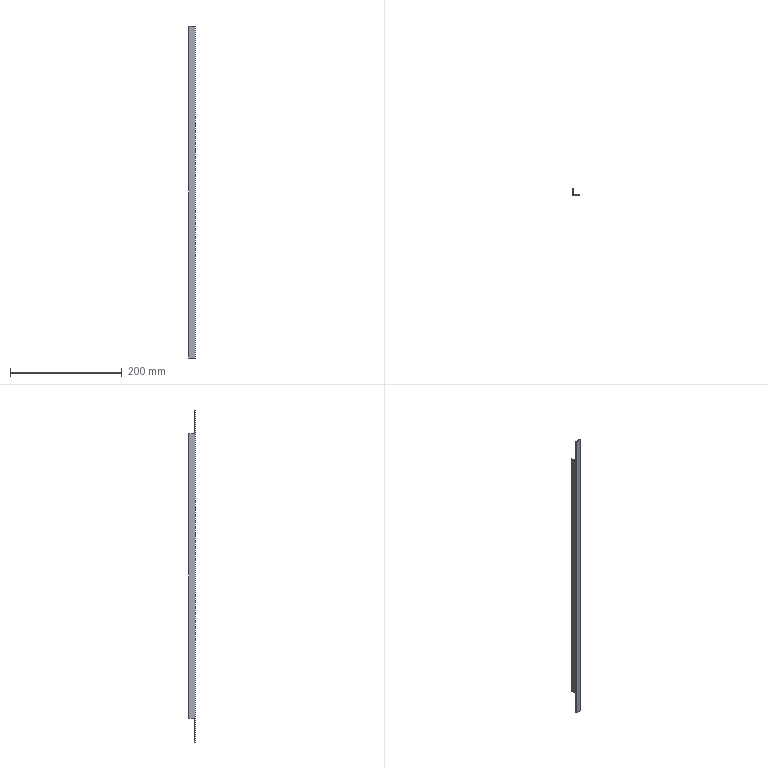Part | SolidWorks | features BaseBody 1 | 1 solid | 20 faces | box 12 x 12 x 594.4 mm | volume 15126 mm3 | plane 14 | cylinder 6 | commonest cylinder face diameters 0.6 x4 1 x2
STEP:
#1=CARTESIAN_POINT('',(1.2,1.7,297.2));
#2=VERTEX_POINT('',#1);
#3=CARTESIAN_POINT('',(1.7,1.2,297.2));
#4=VERTEX_POINT('',#3);
#5=CARTESIAN_POINT('',(1.7,1.7,297.2));
#6=DIRECTION('',(0.,0.,1.));
#7=DIRECTION('',(-1.,0.,0.));
#8=AXIS2_PLACEMENT_3D('',#5,#6,#7);
#9=CIRCLE('',#8,0.5);
#10=EDGE_CURVE('',#2,#4,#9,.T.);
#11=ORIENTED_EDGE('',*,*,#10,.T.);
#12=CARTESIAN_POINT('',(1.7,1.2,-297.2));
#13=VERTEX_POINT('',#12);
#14=CARTESIAN_POINT('',(1.7,1.2,0.));
#15=DIRECTION('',(0.,0.,-1.));
#16=VECTOR('',#15,1000.);
#17=LINE('',#14,#16);
#18=EDGE_CURVE('',#4,#13,#17,.T.);
#19=ORIENTED_EDGE('',*,*,#18,.T.);
#20=CARTESIAN_POINT('',(1.2,1.7,-297.2));
#21=VERTEX_POINT('',#20);
#22=CARTESIAN_POINT('',(1.7,1.7,-297.2));
#23=DIRECTION('',(0.,0.,1.));
#24=DIRECTION('',(-1.,0.,0.));
#25=AXIS2_PLACEMENT_3D('',#22,#23,#24);
#26=CIRCLE('',#25,0.5);
#27=EDGE_CURVE('',#21,#13,#26,.T.);
#28=ORIENTED_EDGE('',*,*,#27,.F.);
#29=CARTESIAN_POINT('',(1.2,1.7,-255.));
#30=VERTEX_POINT('',#29);
#31=CARTESIAN_POINT('',(1.2,1.7,0.));
#32=DIRECTION('',(0.,0.,1.));
#33=VECTOR('',#32,1000.);
#34=LINE('',#31,#33);
#35=EDGE_CURVE('',#21,#30,#34,.T.);
#36=ORIENTED_EDGE('',*,*,#35,.T.);
#37=CARTESIAN_POINT('',(1.2,1.7,255.));
#38=VERTEX_POINT('',#37);
#39=CARTESIAN_POINT('',(1.2,1.7,0.));
#40=DIRECTION('',(0.,0.,1.));
#41=VECTOR('',#40,1000.);
#42=LINE('',#39,#41);
#43=EDGE_CURVE('',#30,#38,#42,.T.);
#44=ORIENTED_EDGE('',*,*,#43,.T.);
#45=CARTESIAN_POINT('',(1.2,1.7,0.));
#46=DIRECTION('',(0.,0.,1.));
#47=VECTOR('',#46,1000.);
#48=LINE('',#45,#47);
#49=EDGE_CURVE('',#38,#2,#48,.T.);
#50=ORIENTED_EDGE('',*,*,#49,.T.);
#51=EDGE_LOOP('',(#11,#19,#28,#36,#44,#50));
#52=FACE_OUTER_BOUND('',#51,.T.);
#53=CARTESIAN_POINT('',(1.7,1.7,297.2));
#54=DIRECTION('',(0.,0.,-1.));
#55=DIRECTION('',(-1.,0.,0.));
#56=AXIS2_PLACEMENT_3D('',#53,#54,#55);
#57=CYLINDRICAL_SURFACE('',#56,0.5);
#58=ADVANCED_FACE('',(#52),#57,.F.);
#59=ORIENTED_EDGE('',*,*,#18,.F.);
#60=CARTESIAN_POINT('',(11.7,1.2,297.2));
#61=VERTEX_POINT('',#60);
#62=CARTESIAN_POINT('',(6.7,1.2,297.2));
#63=DIRECTION('',(-1.,0.,0.));
#64=VECTOR('',#63,1000.);
#65=LINE('',#62,#64);
#66=EDGE_CURVE('',#61,#4,#65,.T.);
#67=ORIENTED_EDGE('',*,*,#66,.F.);
#68=CARTESIAN_POINT('',(11.7,1.2,-297.2));
#69=VERTEX_POINT('',#68);
#70=CARTESIAN_POINT('',(11.7,1.2,0.));
#71=DIRECTION('',(0.,0.,1.));
#72=VECTOR('',#71,1000.);
#73=LINE('',#70,#72);
#74=EDGE_CURVE('',#69,#61,#73,.T.);
#75=ORIENTED_EDGE('',*,*,#74,.F.);
#76=CARTESIAN_POINT('',(6.7,1.2,-297.2));
#77=DIRECTION('',(1.,0.,0.));
#78=VECTOR('',#77,1000.);
#79=LINE('',#76,#78);
#80=EDGE_CURVE('',#13,#69,#79,.T.);
#81=ORIENTED_EDGE('',*,*,#80,.F.);
#82=EDGE_LOOP('',(#59,#67,#75,#81));
#83=FACE_OUTER_BOUND('',#82,.T.);
#84=CARTESIAN_POINT('',(1.7,1.2,-297.2));
#85=DIRECTION('',(0.,-1.,0.));
#86=DIRECTION('',(1.,0.,0.));
#87=AXIS2_PLACEMENT_3D('',#84,#85,#86);
#88=PLANE('',#87);
#89=ADVANCED_FACE('',(#83),#88,.F.);
#90=CARTESIAN_POINT('',(1.2,1.2,297.2));
#91=VERTEX_POINT('',#90);
#92=CARTESIAN_POINT('',(1.2,1.2,255.));
#93=VERTEX_POINT('',#92);
#94=CARTESIAN_POINT('',(1.2,1.2,276.1));
#95=DIRECTION('',(0.,0.,-1.));
#96=VECTOR('',#95,1000.);
#97=LINE('',#94,#96);
#98=EDGE_CURVE('',#91,#93,#97,.T.);
#99=ORIENTED_EDGE('',*,*,#98,.F.);
#100=CARTESIAN_POINT('',(1.2,1.45,297.2));
#101=DIRECTION('',(0.,-1.,0.));
#102=VECTOR('',#101,1000.);
#103=LINE('',#100,#102);
#104=EDGE_CURVE('',#2,#91,#103,.T.);
#105=ORIENTED_EDGE('',*,*,#104,.F.);
#106=ORIENTED_EDGE('',*,*,#49,.F.);
#107=CARTESIAN_POINT('',(1.2,6.6,255.));
#108=DIRECTION('',(0.,-1.,0.));
#109=VECTOR('',#108,1000.);
#110=LINE('',#107,#109);
#111=EDGE_CURVE('',#38,#93,#110,.T.);
#112=ORIENTED_EDGE('',*,*,#111,.T.);
#113=EDGE_LOOP('',(#99,#105,#106,#112));
#114=FACE_OUTER_BOUND('',#113,.T.);
#115=CARTESIAN_POINT('',(1.2,1.2,255.));
#116=DIRECTION('',(1.,0.,0.));
#117=DIRECTION('',(0.,1.,0.));
#118=AXIS2_PLACEMENT_3D('',#115,#116,#117);
#119=PLANE('',#118);
#120=ADVANCED_FACE('',(#114),#119,.F.);
#121=CARTESIAN_POINT('',(1.2,11.7,-255.));
#122=VERTEX_POINT('',#121);
#123=CARTESIAN_POINT('',(1.2,6.7,-255.));
#124=DIRECTION('',(0.,-1.,0.));
#125=VECTOR('',#124,1000.);
#126=LINE('',#123,#125);
#127=EDGE_CURVE('',#122,#30,#126,.T.);
#128=ORIENTED_EDGE('',*,*,#127,.F.);
#129=CARTESIAN_POINT('',(1.2,11.7,255.));
#130=VERTEX_POINT('',#129);
#131=CARTESIAN_POINT('',(1.2,11.7,0.));
#132=DIRECTION('',(0.,0.,-1.));
#133=VECTOR('',#132,1000.);
#134=LINE('',#131,#133);
#135=EDGE_CURVE('',#130,#122,#134,.T.);
#136=ORIENTED_EDGE('',*,*,#135,.F.);
#137=CARTESIAN_POINT('',(1.2,6.7,255.));
#138=DIRECTION('',(0.,1.,0.));
#139=VECTOR('',#138,1000.);
#140=LINE('',#137,#139);
#141=EDGE_CURVE('',#38,#130,#140,.T.);
#142=ORIENTED_EDGE('',*,*,#141,.F.);
#143=ORIENTED_EDGE('',*,*,#43,.F.);
#144=EDGE_LOOP('',(#128,#136,#142,#143));
#145=FACE_OUTER_BOUND('',#144,.T.);
#146=CARTESIAN_POINT('',(1.2,11.7,-255.));
#147=DIRECTION('',(-1.,0.,0.));
#148=DIRECTION('',(0.,-1.,0.));
#149=AXIS2_PLACEMENT_3D('',#146,#147,#148);
#150=PLANE('',#149);
#151=ADVANCED_FACE('',(#145),#150,.F.);
#152=CARTESIAN_POINT('',(1.2,1.2,-255.));
#153=VERTEX_POINT('',#152);
#154=CARTESIAN_POINT('',(1.2,1.2,-297.2));
#155=VERTEX_POINT('',#154);
#156=CARTESIAN_POINT('',(1.2,1.2,-276.1));
#157=DIRECTION('',(0.,0.,-1.));
#158=VECTOR('',#157,1000.);
#159=LINE('',#156,#158);
#160=EDGE_CURVE('',#153,#155,#159,.T.);
#161=ORIENTED_EDGE('',*,*,#160,.F.);
#162=CARTESIAN_POINT('',(1.2,1.45,-255.));
#163=DIRECTION('',(0.,-1.,0.));
#164=VECTOR('',#163,1000.);
#165=LINE('',#162,#164);
#166=EDGE_CURVE('',#30,#153,#165,.T.);
#167=ORIENTED_EDGE('',*,*,#166,.F.);
#168=ORIENTED_EDGE('',*,*,#35,.F.);
#169=CARTESIAN_POINT('',(1.2,1.45,-297.2));
#170=DIRECTION('',(0.,1.,0.));
#171=VECTOR('',#170,1000.);
#172=LINE('',#169,#171);
#173=EDGE_CURVE('',#155,#21,#172,.T.);
#174=ORIENTED_EDGE('',*,*,#173,.F.);
#175=EDGE_LOOP('',(#161,#167,#168,#174));
#176=FACE_OUTER_BOUND('',#175,.T.);
#177=CARTESIAN_POINT('',(1.2,1.2,-297.2));
#178=DIRECTION('',(1.,0.,0.));
#179=DIRECTION('',(0.,1.,0.));
#180=AXIS2_PLACEMENT_3D('',#177,#178,#179);
#181=PLANE('',#180);
#182=ADVANCED_FACE('',(#176),#181,.F.);
#183=CARTESIAN_POINT('',(0.5,0.,-297.2));
#184=VERTEX_POINT('',#183);
#185=CARTESIAN_POINT('',(0.,0.5,-297.2));
#186=VERTEX_POINT('',#185);
#187=CARTESIAN_POINT('',(0.5,0.5,-297.2));
#188=DIRECTION('',(0.,0.,-1.));
#189=DIRECTION('',(-1.,0.,0.));
#190=AXIS2_PLACEMENT_3D('',#187,#188,#189);
#191=CIRCLE('',#190,0.5);
#192=EDGE_CURVE('',#184,#186,#191,.T.);
#193=ORIENTED_EDGE('',*,*,#192,.T.);
#194=CARTESIAN_POINT('',(0.,1.2,-297.2));
#195=VERTEX_POINT('',#194);
#196=CARTESIAN_POINT('',(0.,6.1,-297.2));
#197=DIRECTION('',(0.,1.,0.));
#198=VECTOR('',#197,1000.);
#199=LINE('',#196,#198);
#200=EDGE_CURVE('',#186,#195,#199,.T.);
#201=ORIENTED_EDGE('',*,*,#200,.T.);
#202=CARTESIAN_POINT('',(6.,1.2,-297.2));
#203=DIRECTION('',(1.,0.,0.));
#204=VECTOR('',#203,1000.);
#205=LINE('',#202,#204);
#206=EDGE_CURVE('',#195,#155,#205,.T.);
#207=ORIENTED_EDGE('',*,*,#206,.T.);
#208=ORIENTED_EDGE('',*,*,#173,.T.);
#209=ORIENTED_EDGE('',*,*,#27,.T.);
#210=ORIENTED_EDGE('',*,*,#80,.T.);
#211=CARTESIAN_POINT('',(12.,0.9,-297.2));
#212=VERTEX_POINT('',#211);
#213=CARTESIAN_POINT('',(11.7,0.9,-297.2));
#214=DIRECTION('',(0.,0.,-1.));
#215=DIRECTION('',(-1.,0.,0.));
#216=AXIS2_PLACEMENT_3D('',#213,#214,#215);
#217=CIRCLE('',#216,0.3);
#218=EDGE_CURVE('',#69,#212,#217,.T.);
#219=ORIENTED_EDGE('',*,*,#218,.T.);
#220=CARTESIAN_POINT('',(12.,0.3,-297.2));
#221=VERTEX_POINT('',#220);
#222=CARTESIAN_POINT('',(12.,0.6,-297.2));
#223=DIRECTION('',(0.,-1.,0.));
#224=VECTOR('',#223,1000.);
#225=LINE('',#222,#224);
#226=EDGE_CURVE('',#212,#221,#225,.T.);
#227=ORIENTED_EDGE('',*,*,#226,.T.);
#228=CARTESIAN_POINT('',(11.7,0.,-297.2));
#229=VERTEX_POINT('',#228);
#230=CARTESIAN_POINT('',(11.7,0.3,-297.2));
#231=DIRECTION('',(0.,0.,-1.));
#232=DIRECTION('',(-1.,0.,0.));
#233=AXIS2_PLACEMENT_3D('',#230,#231,#232);
#234=CIRCLE('',#233,0.3);
#235=EDGE_CURVE('',#221,#229,#234,.T.);
#236=ORIENTED_EDGE('',*,*,#235,.T.);
#237=CARTESIAN_POINT('',(6.,0.,-297.2));
#238=DIRECTION('',(-1.,0.,0.));
#239=VECTOR('',#238,1000.);
#240=LINE('',#237,#239);
#241=EDGE_CURVE('',#229,#184,#240,.T.);
#242=ORIENTED_EDGE('',*,*,#241,.T.);
#243=EDGE_LOOP('',(#193,#201,#207,#208,#209,#210,#219,#227,#236,#242));
#244=FACE_OUTER_BOUND('',#243,.T.);
#245=CARTESIAN_POINT('',(12.,0.,-297.2));
#246=DIRECTION('',(0.,0.,-1.));
#247=DIRECTION('',(-1.,0.,0.));
#248=AXIS2_PLACEMENT_3D('',#245,#246,#247);
#249=PLANE('',#248);
#250=ADVANCED_FACE('',(#244),#249,.T.);
#251=CARTESIAN_POINT('',(0.,1.2,297.2));
#252=VERTEX_POINT('',#251);
#253=CARTESIAN_POINT('',(6.,1.2,297.2));
#254=DIRECTION('',(1.,0.,0.));
#255=VECTOR('',#254,1000.);
#256=LINE('',#253,#255);
#257=EDGE_CURVE('',#252,#91,#256,.T.);
#258=ORIENTED_EDGE('',*,*,#257,.F.);
#259=CARTESIAN_POINT('',(0.,0.5,297.2));
#260=VERTEX_POINT('',#259);
#261=CARTESIAN_POINT('',(0.,6.1,297.2));
#262=DIRECTION('',(0.,-1.,0.));
#263=VECTOR('',#262,1000.);
#264=LINE('',#261,#263);
#265=EDGE_CURVE('',#252,#260,#264,.T.);
#266=ORIENTED_EDGE('',*,*,#265,.T.);
#267=CARTESIAN_POINT('',(0.5,0.,297.2));
#268=VERTEX_POINT('',#267);
#269=CARTESIAN_POINT('',(0.5,0.5,297.2));
#270=DIRECTION('',(0.,0.,1.));
#271=DIRECTION('',(-1.,0.,0.));
#272=AXIS2_PLACEMENT_3D('',#269,#270,#271);
#273=CIRCLE('',#272,0.5);
#274=EDGE_CURVE('',#260,#268,#273,.T.);
#275=ORIENTED_EDGE('',*,*,#274,.T.);
#276=CARTESIAN_POINT('',(11.7,0.,297.2));
#277=VERTEX_POINT('',#276);
#278=CARTESIAN_POINT('',(6.,0.,297.2));
#279=DIRECTION('',(-1.,0.,0.));
#280=VECTOR('',#279,1000.);
#281=LINE('',#278,#280);
#282=EDGE_CURVE('',#277,#268,#281,.T.);
#283=ORIENTED_EDGE('',*,*,#282,.F.);
#284=CARTESIAN_POINT('',(12.,0.3,297.2));
#285=VERTEX_POINT('',#284);
#286=CARTESIAN_POINT('',(11.7,0.3,297.2));
#287=DIRECTION('',(0.,0.,1.));
#288=DIRECTION('',(-1.,0.,0.));
#289=AXIS2_PLACEMENT_3D('',#286,#287,#288);
#290=CIRCLE('',#289,0.3);
#291=EDGE_CURVE('',#277,#285,#290,.T.);
#292=ORIENTED_EDGE('',*,*,#291,.T.);
#293=CARTESIAN_POINT('',(12.,0.9,297.2));
#294=VERTEX_POINT('',#293);
#295=CARTESIAN_POINT('',(12.,0.6,297.2));
#296=DIRECTION('',(0.,1.,0.));
#297=VECTOR('',#296,1000.);
#298=LINE('',#295,#297);
#299=EDGE_CURVE('',#285,#294,#298,.T.);
#300=ORIENTED_EDGE('',*,*,#299,.T.);
#301=CARTESIAN_POINT('',(11.7,0.9,297.2));
#302=DIRECTION('',(0.,0.,-1.));
#303=DIRECTION('',(-1.,0.,0.));
#304=AXIS2_PLACEMENT_3D('',#301,#302,#303);
#305=CIRCLE('',#304,0.3);
#306=EDGE_CURVE('',#61,#294,#305,.T.);
#307=ORIENTED_EDGE('',*,*,#306,.F.);
#308=ORIENTED_EDGE('',*,*,#66,.T.);
#309=ORIENTED_EDGE('',*,*,#10,.F.);
#310=ORIENTED_EDGE('',*,*,#104,.T.);
#311=EDGE_LOOP('',(#258,#266,#275,#283,#292,#300,#307,#308,#309,#310));
#312=FACE_OUTER_BOUND('',#311,.T.);
#313=CARTESIAN_POINT('',(12.,0.,297.2));
#314=DIRECTION('',(0.,0.,-1.));
#315=DIRECTION('',(-1.,0.,0.));
#316=AXIS2_PLACEMENT_3D('',#313,#314,#315);
#317=PLANE('',#316);
#318=ADVANCED_FACE('',(#312),#317,.F.);
#319=ORIENTED_EDGE('',*,*,#74,.T.);
#320=ORIENTED_EDGE('',*,*,#306,.T.);
#321=CARTESIAN_POINT('',(12.,0.9,0.));
#322=DIRECTION('',(0.,0.,1.));
#323=VECTOR('',#322,1000.);
#324=LINE('',#321,#323);
#325=EDGE_CURVE('',#212,#294,#324,.T.);
#326=ORIENTED_EDGE('',*,*,#325,.F.);
#327=ORIENTED_EDGE('',*,*,#218,.F.);
#328=EDGE_LOOP('',(#319,#320,#326,#327));
#329=FACE_OUTER_BOUND('',#328,.T.);
#330=CARTESIAN_POINT('',(11.7,0.9,297.2));
#331=DIRECTION('',(0.,0.,-1.));
#332=DIRECTION('',(-1.,0.,0.));
#333=AXIS2_PLACEMENT_3D('',#330,#331,#332);
#334=CYLINDRICAL_SURFACE('',#333,0.3);
#335=ADVANCED_FACE('',(#329),#334,.T.);
#336=ORIENTED_EDGE('',*,*,#98,.T.);
#337=CARTESIAN_POINT('',(0.,1.2,255.));
#338=VERTEX_POINT('',#337);
#339=CARTESIAN_POINT('',(0.6,1.2,255.));
#340=DIRECTION('',(1.,0.,0.));
#341=VECTOR('',#340,1000.);
#342=LINE('',#339,#341);
#343=EDGE_CURVE('',#338,#93,#342,.T.);
#344=ORIENTED_EDGE('',*,*,#343,.F.);
#345=CARTESIAN_POINT('',(0.,1.2,276.1));
#346=DIRECTION('',(0.,0.,-1.));
#347=VECTOR('',#346,1000.);
#348=LINE('',#345,#347);
#349=EDGE_CURVE('',#252,#338,#348,.T.);
#350=ORIENTED_EDGE('',*,*,#349,.F.);
#351=ORIENTED_EDGE('',*,*,#257,.T.);
#352=EDGE_LOOP('',(#336,#344,#350,#351));
#353=FACE_OUTER_BOUND('',#352,.T.);
#354=CARTESIAN_POINT('',(0.,1.2,255.));
#355=DIRECTION('',(0.,-1.,0.));
#356=DIRECTION('',(1.,0.,0.));
#357=AXIS2_PLACEMENT_3D('',#354,#355,#356);
#358=PLANE('',#357);
#359=ADVANCED_FACE('',(#353),#358,.F.);
#360=ORIENTED_EDGE('',*,*,#166,.T.);
#361=CARTESIAN_POINT('',(0.,1.2,-255.));
#362=VERTEX_POINT('',#361);
#363=CARTESIAN_POINT('',(0.6,1.2,-255.));
#364=DIRECTION('',(1.,0.,0.));
#365=VECTOR('',#364,1000.);
#366=LINE('',#363,#365);
#367=EDGE_CURVE('',#362,#153,#366,.T.);
#368=ORIENTED_EDGE('',*,*,#367,.F.);
#369=CARTESIAN_POINT('',(0.,11.7,-255.));
#370=VERTEX_POINT('',#369);
#371=CARTESIAN_POINT('',(0.,6.6,-255.));
#372=DIRECTION('',(0.,-1.,0.));
#373=VECTOR('',#372,1000.);
#374=LINE('',#371,#373);
#375=EDGE_CURVE('',#370,#362,#374,.T.);
#376=ORIENTED_EDGE('',*,*,#375,.F.);
#377=CARTESIAN_POINT('',(0.3,12.,-255.));
#378=VERTEX_POINT('',#377);
#379=CARTESIAN_POINT('',(0.3,11.7,-255.));
#380=DIRECTION('',(0.,0.,-1.));
#381=DIRECTION('',(-1.,0.,0.));
#382=AXIS2_PLACEMENT_3D('',#379,#380,#381);
#383=CIRCLE('',#382,0.3);
#384=EDGE_CURVE('',#370,#378,#383,.T.);
#385=ORIENTED_EDGE('',*,*,#384,.T.);
#386=CARTESIAN_POINT('',(0.9,12.,-255.));
#387=VERTEX_POINT('',#386);
#388=CARTESIAN_POINT('',(0.6,12.,-255.));
#389=DIRECTION('',(1.,0.,0.));
#390=VECTOR('',#389,1000.);
#391=LINE('',#388,#390);
#392=EDGE_CURVE('',#378,#387,#391,.T.);
#393=ORIENTED_EDGE('',*,*,#392,.T.);
#394=CARTESIAN_POINT('',(0.9,11.7,-255.));
#395=DIRECTION('',(0.,0.,1.));
#396=DIRECTION('',(-1.,0.,0.));
#397=AXIS2_PLACEMENT_3D('',#394,#395,#396);
#398=CIRCLE('',#397,0.3);
#399=EDGE_CURVE('',#122,#387,#398,.T.);
#400=ORIENTED_EDGE('',*,*,#399,.F.);
#401=ORIENTED_EDGE('',*,*,#127,.T.);
#402=EDGE_LOOP('',(#360,#368,#376,#385,#393,#400,#401));
#403=FACE_OUTER_BOUND('',#402,.T.);
#404=CARTESIAN_POINT('',(0.,1.2,-255.));
#405=DIRECTION('',(0.,0.,1.));
#406=DIRECTION('',(1.,0.,0.));
#407=AXIS2_PLACEMENT_3D('',#404,#405,#406);
#408=PLANE('',#407);
#409=ADVANCED_FACE('',(#403),#408,.F.);
#410=ORIENTED_EDGE('',*,*,#399,.T.);
#411=CARTESIAN_POINT('',(0.9,12.,255.));
#412=VERTEX_POINT('',#411);
#413=CARTESIAN_POINT('',(0.9,12.,0.));
#414=DIRECTION('',(0.,0.,-1.));
#415=VECTOR('',#414,1000.);
#416=LINE('',#413,#415);
#417=EDGE_CURVE('',#412,#387,#416,.T.);
#418=ORIENTED_EDGE('',*,*,#417,.F.);
#419=CARTESIAN_POINT('',(0.9,11.7,255.));
#420=DIRECTION('',(0.,0.,1.));
#421=DIRECTION('',(-1.,0.,0.));
#422=AXIS2_PLACEMENT_3D('',#419,#420,#421);
#423=CIRCLE('',#422,0.3);
#424=EDGE_CURVE('',#130,#412,#423,.T.);
#425=ORIENTED_EDGE('',*,*,#424,.F.);
#426=ORIENTED_EDGE('',*,*,#135,.T.);
#427=EDGE_LOOP('',(#410,#418,#425,#426));
#428=FACE_OUTER_BOUND('',#427,.T.);
#429=CARTESIAN_POINT('',(0.9,11.7,255.));
#430=DIRECTION('',(0.,0.,-1.));
#431=DIRECTION('',(-1.,0.,0.));
#432=AXIS2_PLACEMENT_3D('',#429,#430,#431);
#433=CYLINDRICAL_SURFACE('',#432,0.3);
#434=ADVANCED_FACE('',(#428),#433,.T.);
#435=CARTESIAN_POINT('',(0.3,12.,255.));
#436=VERTEX_POINT('',#435);
#437=CARTESIAN_POINT('',(0.,11.7,255.));
#438=VERTEX_POINT('',#437);
#439=CARTESIAN_POINT('',(0.3,11.7,255.));
#440=DIRECTION('',(0.,0.,1.));
#441=DIRECTION('',(-1.,0.,0.));
#442=AXIS2_PLACEMENT_3D('',#439,#440,#441);
#443=CIRCLE('',#442,0.3);
#444=EDGE_CURVE('',#436,#438,#443,.T.);
#445=ORIENTED_EDGE('',*,*,#444,.T.);
#446=CARTESIAN_POINT('',(0.,6.6,255.));
#447=DIRECTION('',(0.,1.,0.));
#448=VECTOR('',#447,1000.);
#449=LINE('',#446,#448);
#450=EDGE_CURVE('',#338,#438,#449,.T.);
#451=ORIENTED_EDGE('',*,*,#450,.F.);
#452=ORIENTED_EDGE('',*,*,#343,.T.);
#453=ORIENTED_EDGE('',*,*,#111,.F.);
#454=ORIENTED_EDGE('',*,*,#141,.T.);
#455=ORIENTED_EDGE('',*,*,#424,.T.);
#456=CARTESIAN_POINT('',(0.6,12.,255.));
#457=DIRECTION('',(1.,0.,0.));
#458=VECTOR('',#457,1000.);
#459=LINE('',#456,#458);
#460=EDGE_CURVE('',#436,#412,#459,.T.);
#461=ORIENTED_EDGE('',*,*,#460,.F.);
#462=EDGE_LOOP('',(#445,#451,#452,#453,#454,#455,#461));
#463=FACE_OUTER_BOUND('',#462,.T.);
#464=CARTESIAN_POINT('',(1.2,1.2,255.));
#465=DIRECTION('',(0.,0.,-1.));
#466=DIRECTION('',(-1.,0.,0.));
#467=AXIS2_PLACEMENT_3D('',#464,#465,#466);
#468=PLANE('',#467);
#469=ADVANCED_FACE('',(#463),#468,.F.);
#470=ORIENTED_EDGE('',*,*,#160,.T.);
#471=ORIENTED_EDGE('',*,*,#206,.F.);
#472=CARTESIAN_POINT('',(0.,1.2,-276.1));
#473=DIRECTION('',(0.,0.,-1.));
#474=VECTOR('',#473,1000.);
#475=LINE('',#472,#474);
#476=EDGE_CURVE('',#362,#195,#475,.T.);
#477=ORIENTED_EDGE('',*,*,#476,.F.);
#478=ORIENTED_EDGE('',*,*,#367,.T.);
#479=EDGE_LOOP('',(#470,#471,#477,#478));
#480=FACE_OUTER_BOUND('',#479,.T.);
#481=CARTESIAN_POINT('',(0.,1.2,-297.2));
#482=DIRECTION('',(0.,-1.,0.));
#483=DIRECTION('',(1.,0.,0.));
#484=AXIS2_PLACEMENT_3D('',#481,#482,#483);
#485=PLANE('',#484);
#486=ADVANCED_FACE('',(#480),#485,.F.);
#487=CARTESIAN_POINT('',(11.7,0.,0.));
#488=DIRECTION('',(0.,0.,-1.));
#489=VECTOR('',#488,1000.);
#490=LINE('',#487,#489);
#491=EDGE_CURVE('',#277,#229,#490,.T.);
#492=ORIENTED_EDGE('',*,*,#491,.F.);
#493=ORIENTED_EDGE('',*,*,#282,.T.);
#494=CARTESIAN_POINT('',(0.5,0.,0.));
#495=DIRECTION('',(0.,0.,1.));
#496=VECTOR('',#495,1000.);
#497=LINE('',#494,#496);
#498=EDGE_CURVE('',#184,#268,#497,.T.);
#499=ORIENTED_EDGE('',*,*,#498,.F.);
#500=ORIENTED_EDGE('',*,*,#241,.F.);
#501=EDGE_LOOP('',(#492,#493,#499,#500));
#502=FACE_OUTER_BOUND('',#501,.T.);
#503=CARTESIAN_POINT('',(0.5,0.,-297.2));
#504=DIRECTION('',(0.,1.,0.));
#505=DIRECTION('',(0.,0.,1.));
#506=AXIS2_PLACEMENT_3D('',#503,#504,#505);
#507=PLANE('',#506);
#508=ADVANCED_FACE('',(#502),#507,.F.);
#509=ORIENTED_EDGE('',*,*,#325,.T.);
#510=ORIENTED_EDGE('',*,*,#299,.F.);
#511=CARTESIAN_POINT('',(12.,0.3,0.));
#512=DIRECTION('',(0.,0.,1.));
#513=VECTOR('',#512,1000.);
#514=LINE('',#511,#513);
#515=EDGE_CURVE('',#221,#285,#514,.T.);
#516=ORIENTED_EDGE('',*,*,#515,.F.);
#517=ORIENTED_EDGE('',*,*,#226,.F.);
#518=EDGE_LOOP('',(#509,#510,#516,#517));
#519=FACE_OUTER_BOUND('',#518,.T.);
#520=CARTESIAN_POINT('',(12.,0.3,-297.2));
#521=DIRECTION('',(-1.,0.,0.));
#522=DIRECTION('',(0.,0.,1.));
#523=AXIS2_PLACEMENT_3D('',#520,#521,#522);
#524=PLANE('',#523);
#525=ADVANCED_FACE('',(#519),#524,.F.);
#526=ORIENTED_EDGE('',*,*,#375,.T.);
#527=ORIENTED_EDGE('',*,*,#476,.T.);
#528=ORIENTED_EDGE('',*,*,#200,.F.);
#529=CARTESIAN_POINT('',(0.,0.5,0.));
#530=DIRECTION('',(0.,0.,-1.));
#531=VECTOR('',#530,1000.);
#532=LINE('',#529,#531);
#533=EDGE_CURVE('',#260,#186,#532,.T.);
#534=ORIENTED_EDGE('',*,*,#533,.F.);
#535=ORIENTED_EDGE('',*,*,#265,.F.);
#536=ORIENTED_EDGE('',*,*,#349,.T.);
#537=ORIENTED_EDGE('',*,*,#450,.T.);
#538=CARTESIAN_POINT('',(0.,11.7,0.));
#539=DIRECTION('',(0.,0.,1.));
#540=VECTOR('',#539,1000.);
#541=LINE('',#538,#540);
#542=EDGE_CURVE('',#370,#438,#541,.T.);
#543=ORIENTED_EDGE('',*,*,#542,.F.);
#544=EDGE_LOOP('',(#526,#527,#528,#534,#535,#536,#537,#543));
#545=FACE_OUTER_BOUND('',#544,.T.);
#546=CARTESIAN_POINT('',(0.,0.5,297.2));
#547=DIRECTION('',(1.,0.,0.));
#548=DIRECTION('',(0.,0.,-1.));
#549=AXIS2_PLACEMENT_3D('',#546,#547,#548);
#550=PLANE('',#549);
#551=ADVANCED_FACE('',(#545),#550,.F.);
#552=ORIENTED_EDGE('',*,*,#392,.F.);
#553=CARTESIAN_POINT('',(0.3,12.,0.));
#554=DIRECTION('',(0.,0.,-1.));
#555=VECTOR('',#554,1000.);
#556=LINE('',#553,#555);
#557=EDGE_CURVE('',#436,#378,#556,.T.);
#558=ORIENTED_EDGE('',*,*,#557,.F.);
#559=ORIENTED_EDGE('',*,*,#460,.T.);
#560=ORIENTED_EDGE('',*,*,#417,.T.);
#561=EDGE_LOOP('',(#552,#558,#559,#560));
#562=FACE_OUTER_BOUND('',#561,.T.);
#563=CARTESIAN_POINT('',(0.3,12.,255.));
#564=DIRECTION('',(0.,-1.,0.));
#565=DIRECTION('',(0.,0.,-1.));
#566=AXIS2_PLACEMENT_3D('',#563,#564,#565);
#567=PLANE('',#566);
#568=ADVANCED_FACE('',(#562),#567,.F.);
#569=ORIENTED_EDGE('',*,*,#515,.T.);
#570=ORIENTED_EDGE('',*,*,#291,.F.);
#571=ORIENTED_EDGE('',*,*,#491,.T.);
#572=ORIENTED_EDGE('',*,*,#235,.F.);
#573=EDGE_LOOP('',(#569,#570,#571,#572));
#574=FACE_OUTER_BOUND('',#573,.T.);
#575=CARTESIAN_POINT('',(11.7,0.3,297.2));
#576=DIRECTION('',(0.,0.,-1.));
#577=DIRECTION('',(-1.,0.,0.));
#578=AXIS2_PLACEMENT_3D('',#575,#576,#577);
#579=CYLINDRICAL_SURFACE('',#578,0.3);
#580=ADVANCED_FACE('',(#574),#579,.T.);
#581=ORIENTED_EDGE('',*,*,#498,.T.);
#582=ORIENTED_EDGE('',*,*,#274,.F.);
#583=ORIENTED_EDGE('',*,*,#533,.T.);
#584=ORIENTED_EDGE('',*,*,#192,.F.);
#585=EDGE_LOOP('',(#581,#582,#583,#584));
#586=FACE_OUTER_BOUND('',#585,.T.);
#587=CARTESIAN_POINT('',(0.5,0.5,297.2));
#588=DIRECTION('',(0.,0.,-1.));
#589=DIRECTION('',(-1.,0.,0.));
#590=AXIS2_PLACEMENT_3D('',#587,#588,#589);
#591=CYLINDRICAL_SURFACE('',#590,0.5);
#592=ADVANCED_FACE('',(#586),#591,.T.);
#593=ORIENTED_EDGE('',*,*,#384,.F.);
#594=ORIENTED_EDGE('',*,*,#542,.T.);
#595=ORIENTED_EDGE('',*,*,#444,.F.);
#596=ORIENTED_EDGE('',*,*,#557,.T.);
#597=EDGE_LOOP('',(#593,#594,#595,#596));
#598=FACE_OUTER_BOUND('',#597,.T.);
#599=CARTESIAN_POINT('',(0.3,11.7,255.));
#600=DIRECTION('',(0.,0.,-1.));
#601=DIRECTION('',(-1.,0.,0.));
#602=AXIS2_PLACEMENT_3D('',#599,#600,#601);
#603=CYLINDRICAL_SURFACE('',#602,0.3);
#604=ADVANCED_FACE('',(#598),#603,.T.);
#605=CLOSED_SHELL('',(#58,#89,#120,#151,#182,#250,#318,#335,#359,#409,#434,#469,#486,#508,#525,#551,#568,#580,#592,#604));
#606=MANIFOLD_SOLID_BREP('',#605);
#607=CARTESIAN_POINT('',(0.,0.,0.));
#608=DIRECTION('',(0.,0.,1.));
#609=DIRECTION('',(1.,0.,0.));
#610=AXIS2_PLACEMENT_3D('',#607,#608,#609);
#611=(LENGTH_UNIT()NAMED_UNIT(*)SI_UNIT(.MILLI.,.METRE.));
#612=UNCERTAINTY_MEASURE_WITH_UNIT(LENGTH_MEASURE(0.00001),#611,'','');
#613=(NAMED_UNIT(*)PLANE_ANGLE_UNIT()SI_UNIT($,.RADIAN.));
#614=(NAMED_UNIT(*)SI_UNIT($,.STERADIAN.)SOLID_ANGLE_UNIT());
#615=(GEOMETRIC_REPRESENTATION_CONTEXT(3)GLOBAL_UNCERTAINTY_ASSIGNED_CONTEXT((#612))GLOBAL_UNIT_ASSIGNED_CONTEXT((#611,#613,#614))REPRESENTATION_CONTEXT('',''));
#616=ADVANCED_BREP_SHAPE_REPRESENTATION('',(#606,#610),#615);